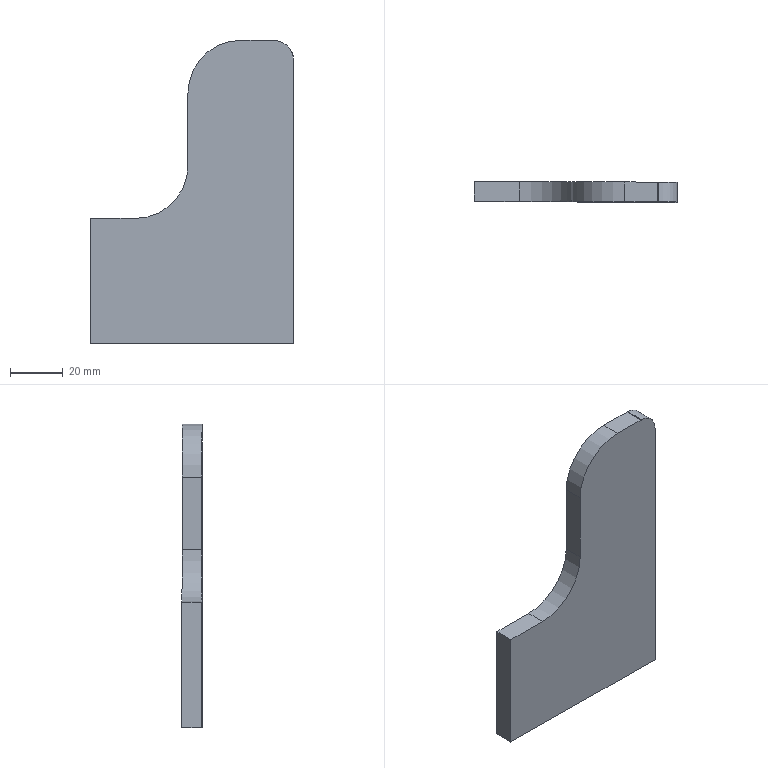Part | STEP file | 2026.6.15-Main Assembly图.sldasm-Part-145 | 1 solid | 12 faces | box 77.037 x 7.893 x 115 mm | volume 47591 mm3 | plane 8 | cylinder 4 | commonest cylinder face diameters 15 x2 40 x2
STEP:
#1=CARTESIAN_POINT('',(-1540.308,1364.174,3792.567));
#2=VERTEX_POINT('',#1);
#3=CARTESIAN_POINT('',(-1540.56,1364.175,3792.571));
#4=VERTEX_POINT('',#3);
#5=CARTESIAN_POINT('',(-1540.56,1364.175,3785.071));
#6=DIRECTION('',(-0.005111,-1.,0.));
#7=DIRECTION('',(-1.,0.005111,0.));
#8=AXIS2_PLACEMENT_3D('',#5,#6,#7);
#9=CIRCLE('',#8,7.5);
#10=EDGE_CURVE('',#2,#4,#9,.T.);
#11=ORIENTED_EDGE('',*,*,#10,.F.);
#12=CARTESIAN_POINT('',(-1540.27,1371.674,3792.567));
#13=VERTEX_POINT('',#12);
#14=CARTESIAN_POINT('',(-1540.308,1364.174,3792.567));
#15=DIRECTION('',(0.005111,1.,0.));
#16=VECTOR('',#15,1000.);
#17=LINE('',#14,#16);
#18=EDGE_CURVE('',#2,#13,#17,.T.);
#19=ORIENTED_EDGE('',*,*,#18,.T.);
#20=CARTESIAN_POINT('',(-1540.521,1371.675,3792.571));
#21=VERTEX_POINT('',#20);
#22=CARTESIAN_POINT('',(-1540.521,1371.675,3785.071));
#23=DIRECTION('',(-0.005111,-1.,0.));
#24=DIRECTION('',(-1.,0.005111,0.));
#25=AXIS2_PLACEMENT_3D('',#22,#23,#24);
#26=CIRCLE('',#25,7.5);
#27=EDGE_CURVE('',#13,#21,#26,.T.);
#28=ORIENTED_EDGE('',*,*,#27,.T.);
#29=CARTESIAN_POINT('',(-1540.56,1364.175,3792.571));
#30=DIRECTION('',(0.005111,1.,0.));
#31=VECTOR('',#30,1000.);
#32=LINE('',#29,#31);
#33=EDGE_CURVE('',#4,#21,#32,.T.);
#34=ORIENTED_EDGE('',*,*,#33,.F.);
#35=EDGE_LOOP('',(#11,#19,#28,#34));
#36=FACE_OUTER_BOUND('',#35,.T.);
#37=CARTESIAN_POINT('',(-1540.56,1364.175,3785.071));
#38=DIRECTION('',(0.005111,1.,0.));
#39=DIRECTION('',(0.03353,-0.0001714,0.9994));
#40=AXIS2_PLACEMENT_3D('',#37,#38,#39);
#41=CYLINDRICAL_SURFACE('',#40,7.5);
#42=ADVANCED_FACE('',(#36),#41,.T.);
#43=CARTESIAN_POINT('',(-1610.021,1372.031,3677.571));
#44=VERTEX_POINT('',#43);
#45=CARTESIAN_POINT('',(-1533.022,1371.637,3677.571));
#46=VERTEX_POINT('',#45);
#47=CARTESIAN_POINT('',(-1610.021,1372.031,3677.571));
#48=DIRECTION('',(1.,-0.005111,0.));
#49=VECTOR('',#48,1000.);
#50=LINE('',#47,#49);
#51=EDGE_CURVE('',#44,#46,#50,.T.);
#52=ORIENTED_EDGE('',*,*,#51,.T.);
#53=CARTESIAN_POINT('',(-1533.06,1364.137,3677.571));
#54=VERTEX_POINT('',#53);
#55=CARTESIAN_POINT('',(-1533.06,1364.137,3677.571));
#56=DIRECTION('',(0.005111,1.,0.));
#57=VECTOR('',#56,1000.);
#58=LINE('',#55,#57);
#59=EDGE_CURVE('',#54,#46,#58,.T.);
#60=ORIENTED_EDGE('',*,*,#59,.F.);
#61=CARTESIAN_POINT('',(-1610.059,1364.531,3677.571));
#62=VERTEX_POINT('',#61);
#63=CARTESIAN_POINT('',(-1610.059,1364.531,3677.571));
#64=DIRECTION('',(1.,-0.005111,0.));
#65=VECTOR('',#64,1000.);
#66=LINE('',#63,#65);
#67=EDGE_CURVE('',#62,#54,#66,.T.);
#68=ORIENTED_EDGE('',*,*,#67,.F.);
#69=CARTESIAN_POINT('',(-1610.059,1364.531,3677.571));
#70=DIRECTION('',(0.005111,1.,0.));
#71=VECTOR('',#70,1000.);
#72=LINE('',#69,#71);
#73=EDGE_CURVE('',#62,#44,#72,.T.);
#74=ORIENTED_EDGE('',*,*,#73,.T.);
#75=EDGE_LOOP('',(#52,#60,#68,#74));
#76=FACE_OUTER_BOUND('',#75,.T.);
#77=CARTESIAN_POINT('',(-1610.059,1364.531,3677.571));
#78=DIRECTION('',(0.,0.,1.));
#79=DIRECTION('',(-0.0007664,-1.,0.));
#80=AXIS2_PLACEMENT_3D('',#77,#78,#79);
#81=PLANE('',#80);
#82=ADVANCED_FACE('',(#76),#81,.F.);
#83=CARTESIAN_POINT('',(-1533.022,1371.637,3785.071));
#84=VERTEX_POINT('',#83);
#85=CARTESIAN_POINT('',(-1533.022,1371.637,3677.571));
#86=DIRECTION('',(0.,0.,1.));
#87=VECTOR('',#86,1000.);
#88=LINE('',#85,#87);
#89=EDGE_CURVE('',#46,#84,#88,.T.);
#90=ORIENTED_EDGE('',*,*,#89,.T.);
#91=CARTESIAN_POINT('',(-1533.06,1364.137,3785.071));
#92=VERTEX_POINT('',#91);
#93=CARTESIAN_POINT('',(-1533.06,1364.137,3785.071));
#94=DIRECTION('',(0.005111,1.,0.));
#95=VECTOR('',#94,1000.);
#96=LINE('',#93,#95);
#97=EDGE_CURVE('',#92,#84,#96,.T.);
#98=ORIENTED_EDGE('',*,*,#97,.F.);
#99=CARTESIAN_POINT('',(-1533.06,1364.137,3677.571));
#100=DIRECTION('',(0.,0.,1.));
#101=VECTOR('',#100,1000.);
#102=LINE('',#99,#101);
#103=EDGE_CURVE('',#54,#92,#102,.T.);
#104=ORIENTED_EDGE('',*,*,#103,.F.);
#105=ORIENTED_EDGE('',*,*,#59,.T.);
#106=EDGE_LOOP('',(#90,#98,#104,#105));
#107=FACE_OUTER_BOUND('',#106,.T.);
#108=CARTESIAN_POINT('',(-1533.06,1364.137,3677.571));
#109=DIRECTION('',(-1.,0.005111,0.));
#110=DIRECTION('',(-0.0006563,-0.1284,0.9917));
#111=AXIS2_PLACEMENT_3D('',#108,#109,#110);
#112=PLANE('',#111);
#113=ADVANCED_FACE('',(#107),#112,.F.);
#114=ORIENTED_EDGE('',*,*,#18,.F.);
#115=CARTESIAN_POINT('',(-1540.56,1364.175,3785.071));
#116=DIRECTION('',(-0.005111,-1.,0.));
#117=DIRECTION('',(-1.,0.005111,0.));
#118=AXIS2_PLACEMENT_3D('',#115,#116,#117);
#119=CIRCLE('',#118,7.5);
#120=EDGE_CURVE('',#92,#2,#119,.T.);
#121=ORIENTED_EDGE('',*,*,#120,.F.);
#122=ORIENTED_EDGE('',*,*,#97,.T.);
#123=CARTESIAN_POINT('',(-1540.521,1371.675,3785.071));
#124=DIRECTION('',(-0.005111,-1.,0.));
#125=DIRECTION('',(-1.,0.005111,0.));
#126=AXIS2_PLACEMENT_3D('',#123,#124,#125);
#127=CIRCLE('',#126,7.5);
#128=EDGE_CURVE('',#84,#13,#127,.T.);
#129=ORIENTED_EDGE('',*,*,#128,.T.);
#130=EDGE_LOOP('',(#114,#121,#122,#129));
#131=FACE_OUTER_BOUND('',#130,.T.);
#132=CARTESIAN_POINT('',(-1540.56,1364.175,3785.071));
#133=DIRECTION('',(0.005111,1.,0.));
#134=DIRECTION('',(0.03353,-0.0001714,0.9994));
#135=AXIS2_PLACEMENT_3D('',#132,#133,#134);
#136=CYLINDRICAL_SURFACE('',#135,7.5);
#137=ADVANCED_FACE('',(#131),#136,.T.);
#138=CARTESIAN_POINT('',(-1553.021,1371.739,3792.571));
#139=VERTEX_POINT('',#138);
#140=CARTESIAN_POINT('',(-1540.521,1371.675,3792.571));
#141=DIRECTION('',(-1.,0.005111,0.));
#142=VECTOR('',#141,1000.);
#143=LINE('',#140,#142);
#144=EDGE_CURVE('',#21,#139,#143,.T.);
#145=ORIENTED_EDGE('',*,*,#144,.T.);
#146=CARTESIAN_POINT('',(-1553.06,1364.239,3792.571));
#147=VERTEX_POINT('',#146);
#148=CARTESIAN_POINT('',(-1553.06,1364.239,3792.571));
#149=DIRECTION('',(0.005111,1.,0.));
#150=VECTOR('',#149,1000.);
#151=LINE('',#148,#150);
#152=EDGE_CURVE('',#147,#139,#151,.T.);
#153=ORIENTED_EDGE('',*,*,#152,.F.);
#154=CARTESIAN_POINT('',(-1540.56,1364.175,3792.571));
#155=DIRECTION('',(-1.,0.005111,0.));
#156=VECTOR('',#155,1000.);
#157=LINE('',#154,#156);
#158=EDGE_CURVE('',#4,#147,#157,.T.);
#159=ORIENTED_EDGE('',*,*,#158,.F.);
#160=ORIENTED_EDGE('',*,*,#33,.T.);
#161=EDGE_LOOP('',(#145,#153,#159,#160));
#162=FACE_OUTER_BOUND('',#161,.T.);
#163=CARTESIAN_POINT('',(-1540.56,1364.175,3792.571));
#164=DIRECTION('',(0.,0.,-1.));
#165=DIRECTION('',(0.0007664,1.,0.));
#166=AXIS2_PLACEMENT_3D('',#163,#164,#165);
#167=PLANE('',#166);
#168=ADVANCED_FACE('',(#162),#167,.F.);
#169=CARTESIAN_POINT('',(-1573.021,1371.841,3772.571));
#170=VERTEX_POINT('',#169);
#171=CARTESIAN_POINT('',(-1553.021,1371.739,3772.571));
#172=DIRECTION('',(-0.005111,-1.,0.));
#173=DIRECTION('',(-1.,0.005111,0.));
#174=AXIS2_PLACEMENT_3D('',#171,#172,#173);
#175=CIRCLE('',#174,20.);
#176=EDGE_CURVE('',#139,#170,#175,.T.);
#177=ORIENTED_EDGE('',*,*,#176,.T.);
#178=CARTESIAN_POINT('',(-1573.059,1364.342,3772.571));
#179=VERTEX_POINT('',#178);
#180=CARTESIAN_POINT('',(-1573.059,1364.342,3772.571));
#181=DIRECTION('',(0.005111,1.,0.));
#182=VECTOR('',#181,1000.);
#183=LINE('',#180,#182);
#184=EDGE_CURVE('',#179,#170,#183,.T.);
#185=ORIENTED_EDGE('',*,*,#184,.F.);
#186=CARTESIAN_POINT('',(-1553.06,1364.239,3772.571));
#187=DIRECTION('',(-0.005111,-1.,0.));
#188=DIRECTION('',(-1.,0.005111,0.));
#189=AXIS2_PLACEMENT_3D('',#186,#187,#188);
#190=CIRCLE('',#189,20.);
#191=EDGE_CURVE('',#147,#179,#190,.T.);
#192=ORIENTED_EDGE('',*,*,#191,.F.);
#193=ORIENTED_EDGE('',*,*,#152,.T.);
#194=EDGE_LOOP('',(#177,#185,#192,#193));
#195=FACE_OUTER_BOUND('',#194,.T.);
#196=CARTESIAN_POINT('',(-1553.06,1364.239,3772.571));
#197=DIRECTION('',(0.005111,1.,0.));
#198=DIRECTION('',(0.03353,-0.0001714,0.9994));
#199=AXIS2_PLACEMENT_3D('',#196,#197,#198);
#200=CYLINDRICAL_SURFACE('',#199,20.);
#201=ADVANCED_FACE('',(#195),#200,.T.);
#202=CARTESIAN_POINT('',(-1573.021,1371.841,3745.071));
#203=VERTEX_POINT('',#202);
#204=CARTESIAN_POINT('',(-1573.021,1371.841,3772.571));
#205=DIRECTION('',(0.,0.,-1.));
#206=VECTOR('',#205,1000.);
#207=LINE('',#204,#206);
#208=EDGE_CURVE('',#170,#203,#207,.T.);
#209=ORIENTED_EDGE('',*,*,#208,.T.);
#210=CARTESIAN_POINT('',(-1573.059,1364.342,3745.071));
#211=VERTEX_POINT('',#210);
#212=CARTESIAN_POINT('',(-1573.059,1364.342,3745.071));
#213=DIRECTION('',(0.005111,1.,0.));
#214=VECTOR('',#213,1000.);
#215=LINE('',#212,#214);
#216=EDGE_CURVE('',#211,#203,#215,.T.);
#217=ORIENTED_EDGE('',*,*,#216,.F.);
#218=CARTESIAN_POINT('',(-1573.059,1364.342,3772.571));
#219=DIRECTION('',(0.,0.,-1.));
#220=VECTOR('',#219,1000.);
#221=LINE('',#218,#220);
#222=EDGE_CURVE('',#179,#211,#221,.T.);
#223=ORIENTED_EDGE('',*,*,#222,.F.);
#224=ORIENTED_EDGE('',*,*,#184,.T.);
#225=EDGE_LOOP('',(#209,#217,#223,#224));
#226=FACE_OUTER_BOUND('',#225,.T.);
#227=CARTESIAN_POINT('',(-1573.059,1364.342,3772.571));
#228=DIRECTION('',(1.,-0.005111,0.));
#229=DIRECTION('',(0.0006563,0.1284,-0.9917));
#230=AXIS2_PLACEMENT_3D('',#227,#228,#229);
#231=PLANE('',#230);
#232=ADVANCED_FACE('',(#226),#231,.F.);
#233=CARTESIAN_POINT('',(-1593.021,1371.944,3725.071));
#234=VERTEX_POINT('',#233);
#235=CARTESIAN_POINT('',(-1593.021,1371.944,3745.071));
#236=DIRECTION('',(0.005111,1.,0.));
#237=DIRECTION('',(-1.,0.005111,0.));
#238=AXIS2_PLACEMENT_3D('',#235,#236,#237);
#239=CIRCLE('',#238,20.);
#240=EDGE_CURVE('',#203,#234,#239,.T.);
#241=ORIENTED_EDGE('',*,*,#240,.T.);
#242=CARTESIAN_POINT('',(-1593.059,1364.444,3725.071));
#243=VERTEX_POINT('',#242);
#244=CARTESIAN_POINT('',(-1593.059,1364.444,3725.071));
#245=DIRECTION('',(0.005111,1.,0.));
#246=VECTOR('',#245,1000.);
#247=LINE('',#244,#246);
#248=EDGE_CURVE('',#243,#234,#247,.T.);
#249=ORIENTED_EDGE('',*,*,#248,.F.);
#250=CARTESIAN_POINT('',(-1593.059,1364.444,3745.071));
#251=DIRECTION('',(0.005111,1.,0.));
#252=DIRECTION('',(-1.,0.005111,0.));
#253=AXIS2_PLACEMENT_3D('',#250,#251,#252);
#254=CIRCLE('',#253,20.);
#255=EDGE_CURVE('',#211,#243,#254,.T.);
#256=ORIENTED_EDGE('',*,*,#255,.F.);
#257=ORIENTED_EDGE('',*,*,#216,.T.);
#258=EDGE_LOOP('',(#241,#249,#256,#257));
#259=FACE_OUTER_BOUND('',#258,.T.);
#260=CARTESIAN_POINT('',(-1593.059,1364.444,3745.071));
#261=DIRECTION('',(0.005111,1.,0.));
#262=DIRECTION('',(0.03353,-0.0001714,0.9994));
#263=AXIS2_PLACEMENT_3D('',#260,#261,#262);
#264=CYLINDRICAL_SURFACE('',#263,20.);
#265=ADVANCED_FACE('',(#259),#264,.F.);
#266=CARTESIAN_POINT('',(-1610.021,1372.031,3725.071));
#267=VERTEX_POINT('',#266);
#268=CARTESIAN_POINT('',(-1593.021,1371.944,3725.071));
#269=DIRECTION('',(-1.,0.005111,0.));
#270=VECTOR('',#269,1000.);
#271=LINE('',#268,#270);
#272=EDGE_CURVE('',#234,#267,#271,.T.);
#273=ORIENTED_EDGE('',*,*,#272,.T.);
#274=CARTESIAN_POINT('',(-1610.059,1364.531,3725.071));
#275=VERTEX_POINT('',#274);
#276=CARTESIAN_POINT('',(-1610.059,1364.531,3725.071));
#277=DIRECTION('',(0.005111,1.,0.));
#278=VECTOR('',#277,1000.);
#279=LINE('',#276,#278);
#280=EDGE_CURVE('',#275,#267,#279,.T.);
#281=ORIENTED_EDGE('',*,*,#280,.F.);
#282=CARTESIAN_POINT('',(-1593.059,1364.444,3725.071));
#283=DIRECTION('',(-1.,0.005111,0.));
#284=VECTOR('',#283,1000.);
#285=LINE('',#282,#284);
#286=EDGE_CURVE('',#243,#275,#285,.T.);
#287=ORIENTED_EDGE('',*,*,#286,.F.);
#288=ORIENTED_EDGE('',*,*,#248,.T.);
#289=EDGE_LOOP('',(#273,#281,#287,#288));
#290=FACE_OUTER_BOUND('',#289,.T.);
#291=CARTESIAN_POINT('',(-1593.059,1364.444,3725.071));
#292=DIRECTION('',(0.,0.,-1.));
#293=DIRECTION('',(0.0007664,1.,0.));
#294=AXIS2_PLACEMENT_3D('',#291,#292,#293);
#295=PLANE('',#294);
#296=ADVANCED_FACE('',(#290),#295,.F.);
#297=CARTESIAN_POINT('',(-1610.021,1372.031,3725.071));
#298=DIRECTION('',(0.,0.,-1.));
#299=VECTOR('',#298,1000.);
#300=LINE('',#297,#299);
#301=EDGE_CURVE('',#267,#44,#300,.T.);
#302=ORIENTED_EDGE('',*,*,#301,.T.);
#303=ORIENTED_EDGE('',*,*,#73,.F.);
#304=CARTESIAN_POINT('',(-1610.059,1364.531,3725.071));
#305=DIRECTION('',(0.,0.,-1.));
#306=VECTOR('',#305,1000.);
#307=LINE('',#304,#306);
#308=EDGE_CURVE('',#275,#62,#307,.T.);
#309=ORIENTED_EDGE('',*,*,#308,.F.);
#310=ORIENTED_EDGE('',*,*,#280,.T.);
#311=EDGE_LOOP('',(#302,#303,#309,#310));
#312=FACE_OUTER_BOUND('',#311,.T.);
#313=CARTESIAN_POINT('',(-1610.059,1364.531,3725.071));
#314=DIRECTION('',(1.,-0.005111,0.));
#315=DIRECTION('',(0.0006563,0.1284,-0.9917));
#316=AXIS2_PLACEMENT_3D('',#313,#314,#315);
#317=PLANE('',#316);
#318=ADVANCED_FACE('',(#312),#317,.F.);
#319=ORIENTED_EDGE('',*,*,#67,.T.);
#320=ORIENTED_EDGE('',*,*,#103,.T.);
#321=ORIENTED_EDGE('',*,*,#120,.T.);
#322=ORIENTED_EDGE('',*,*,#10,.T.);
#323=ORIENTED_EDGE('',*,*,#158,.T.);
#324=ORIENTED_EDGE('',*,*,#191,.T.);
#325=ORIENTED_EDGE('',*,*,#222,.T.);
#326=ORIENTED_EDGE('',*,*,#255,.T.);
#327=ORIENTED_EDGE('',*,*,#286,.T.);
#328=ORIENTED_EDGE('',*,*,#308,.T.);
#329=EDGE_LOOP('',(#319,#320,#321,#322,#323,#324,#325,#326,#327,#328));
#330=FACE_OUTER_BOUND('',#329,.T.);
#331=CARTESIAN_POINT('',(-1540.56,1364.175,3785.071));
#332=DIRECTION('',(-0.005111,-1.,0.));
#333=DIRECTION('',(-0.03353,0.0001714,-0.9994));
#334=AXIS2_PLACEMENT_3D('',#331,#332,#333);
#335=PLANE('',#334);
#336=ADVANCED_FACE('',(#330),#335,.T.);
#337=ORIENTED_EDGE('',*,*,#51,.F.);
#338=ORIENTED_EDGE('',*,*,#301,.F.);
#339=ORIENTED_EDGE('',*,*,#272,.F.);
#340=ORIENTED_EDGE('',*,*,#240,.F.);
#341=ORIENTED_EDGE('',*,*,#208,.F.);
#342=ORIENTED_EDGE('',*,*,#176,.F.);
#343=ORIENTED_EDGE('',*,*,#144,.F.);
#344=ORIENTED_EDGE('',*,*,#27,.F.);
#345=ORIENTED_EDGE('',*,*,#128,.F.);
#346=ORIENTED_EDGE('',*,*,#89,.F.);
#347=EDGE_LOOP('',(#337,#338,#339,#340,#341,#342,#343,#344,#345,#346));
#348=FACE_OUTER_BOUND('',#347,.T.);
#349=CARTESIAN_POINT('',(-1540.521,1371.675,3785.071));
#350=DIRECTION('',(-0.005111,-1.,0.));
#351=DIRECTION('',(-0.03353,0.0001714,-0.9994));
#352=AXIS2_PLACEMENT_3D('',#349,#350,#351);
#353=PLANE('',#352);
#354=ADVANCED_FACE('',(#348),#353,.F.);
#355=CLOSED_SHELL('',(#42,#82,#113,#137,#168,#201,#232,#265,#296,#318,#336,#354));
#356=MANIFOLD_SOLID_BREP('',#355);
#357=CARTESIAN_POINT('',(0.,0.,0.));
#358=DIRECTION('',(0.,0.,1.));
#359=DIRECTION('',(1.,0.,0.));
#360=AXIS2_PLACEMENT_3D('',#357,#358,#359);
#361=(LENGTH_UNIT()NAMED_UNIT(*)SI_UNIT(.MILLI.,.METRE.));
#362=UNCERTAINTY_MEASURE_WITH_UNIT(LENGTH_MEASURE(0.00001),#361,'','');
#363=(NAMED_UNIT(*)PLANE_ANGLE_UNIT()SI_UNIT($,.RADIAN.));
#364=(NAMED_UNIT(*)SI_UNIT($,.STERADIAN.)SOLID_ANGLE_UNIT());
#365=(GEOMETRIC_REPRESENTATION_CONTEXT(3)GLOBAL_UNCERTAINTY_ASSIGNED_CONTEXT((#362))GLOBAL_UNIT_ASSIGNED_CONTEXT((#361,#363,#364))REPRESENTATION_CONTEXT('',''));
#366=ADVANCED_BREP_SHAPE_REPRESENTATION('',(#356,#360),#365);